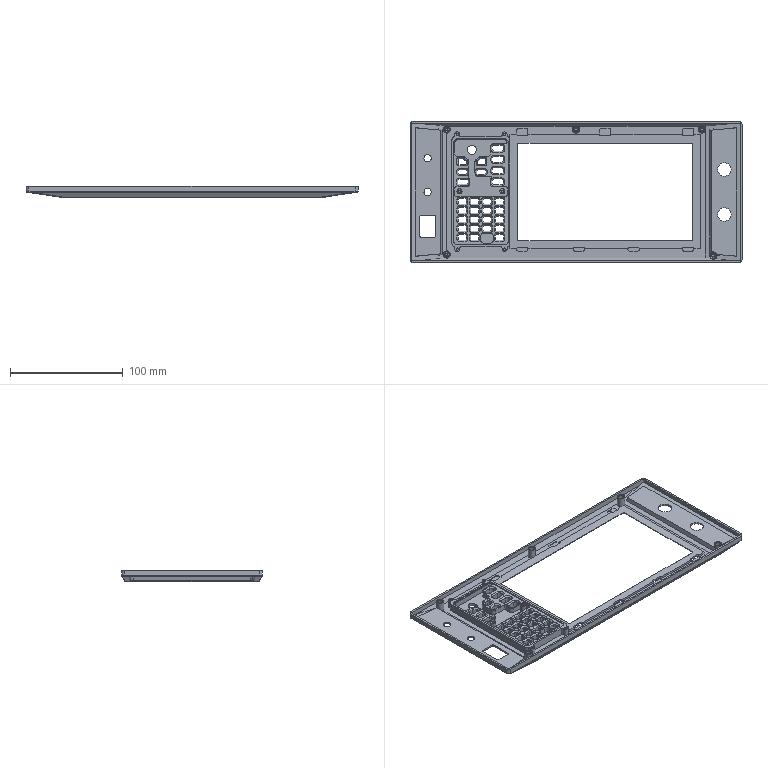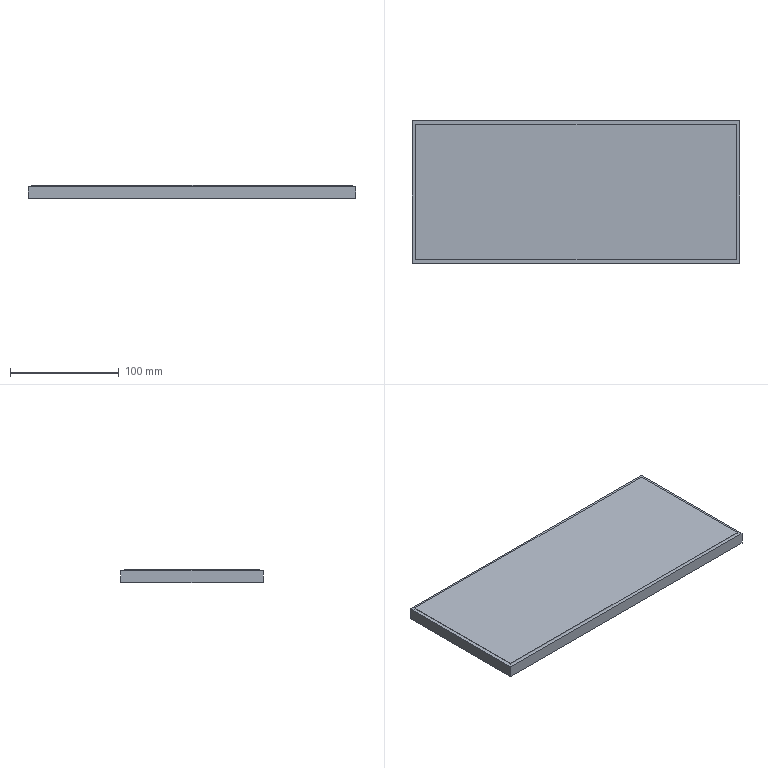CAM job | NX | 3-axis milling, drilling | part box 295 x 125 x 10 mm | stock box 301 x 131 x 12 mm
Tools:
number,name,description,diameter,corner_radius,flute_length,length,flutes
1,D63,Milling Tool-5 Parameters,63.0,0.0,50.0,75.0,2
7,D6A45,Milling Tool-5 Parameters,6.0,0.0,50.0,75.0,2
12,2.5ZT,Drilling Tool,2.5,0.0,35.0,50.0,2
13,2.1ZT,Drilling Tool,2.05,0.0,35.0,50.0,2
10,D10,Milling Tool-5 Parameters,10.0,0.0,50.0,75.0,2
6,D6,Milling Tool-5 Parameters,6.0,0.0,50.0,75.0,2
4,D4,Milling Tool-5 Parameters,4.0,0.0,50.0,75.0,2
2,D2,Milling Tool-5 Parameters,2.0,0.0,50.0,75.0,2
15,D1.5,Milling Tool-5 Parameters,1.5,0.0,50.0,75.0,2
5,D2R0.5,Milling Tool-5 Parameters,2.0,0.5,50.0,75.0,2
9,D6R0.5,Milling Tool-5 Parameters,6.0,0.5,50.0,75.0,2
Operations:
program,operation,operation_type,tool,method,geometry_group,spindle_rpm,surface_speed,feed_per_tooth,feed_cut,feed_plunge,cut_length_mm,path_length_mm,cut_time_min,machine_time_min
1,FLOOR_WALL,VolumeBased25DMillingOperation,D63,METHOD,A,6500.0,1286.0,0.0962,1250.0,100.0,1573.797,1627.797,1.259,1.264
1,DRILLING,Operation,D6A45,METHOD,A,5000.0,94.0,0.025,250.0,0.0,40.0,648.236,0.16,0.2208
1,DRILLING_COPY,Operation,2.5ZT,METHOD,A,2000.0,15.0,0.03,120.0,0.0,42.0,629.23,0.35,0.4087
1,DRILLING_COPY_COPY,Operation,2.1ZT,METHOD,A,2000.0,12.0,0.03,120.0,0.0,63.0,425.557,0.525,0.5613
1,ADAPTIVE_MILLING,CavityMilling,D10,METHOD,A,9500.0,298.0,0.1579,3000.0,1000.0,3506.591,3580.591,1.171,1.178
1,ADAPTIVE_MILLING_COPY,CavityMilling,D10,METHOD,A,9500.0,298.0,0.1579,3000.0,1000.0,26947.709,27013.909,9.563,9.57
1,CAVITY_MILL,CavityMilling,D10,METHOD,A,9500.0,298.0,0.1579,3000.0,1000.0,26927.247,28801.245,10.357,10.545
1,CAVITY_MILL_COPY,CavityMilling,D6,METHOD,A,9500.0,179.0,0.1053,2000.0,1000.0,13061.75,22740.845,8.004,8.972
1,ZLEVEL_PROFILE_COPY_COPY_COPY_1,ZLevelMilling,D6,METHOD,A,9500.0,44.0,0.0526,1000.0,100.0,860.807,937.807,0.8608,0.8685
1,HOLE_MILLING,CylinderMilling,D4,METHOD,A,9500.0,119.0,0.0737,1400.0,100.0,544.282,1273.844,0.3888,0.4617
1,HOLE_MILLING_COPY,CylinderMilling,D4,METHOD,A,9500.0,119.0,0.0526,1000.0,100.0,202.496,932.058,0.2025,0.2755
1,CAVITY_MILL_COPY_COPY,CavityMilling,D4,METHOD,A,9500.0,119.0,0.0868,1650.0,1000.0,30994.875,48438.889,25.426,27.171
1,FLOOR_WALL_1,VolumeBased25DMillingOperation,D4,METHOD,A,9500.0,119.0,0.0526,1000.0,100.0,15303.61,21184.288,15.304,15.892
1,CAVITY_MILL_COPY_COPY_COPY,CavityMilling,D2,METHOD,A,9500.0,59.0,0.0526,1000.0,1000.0,51842.907,83769.591,51.843,55.036
1,HOLE_MILLING_1,CylinderMilling,D2,METHOD,A,9500.0,59.0,0.0579,1100.0,100.0,1184.848,1993.624,1.077,1.158
1,ZLEVEL_PROFILE_COPY_COPY,ZLevelMilling,D2,METHOD,A,9500.0,44.0,0.0526,1000.0,100.0,63.243,131.781,0.0632,0.0701
1,ZLEVEL_PROFILE_COPY_COPY_COPY,ZLevelMilling,D2,METHOD,A,9500.0,44.0,0.0526,1000.0,100.0,609.106,3438.851,0.6091,0.8921
1,ZLEVEL_PROFILE_COPY_COPY_COPY_2,ZLevelMilling,D2,METHOD,A,9500.0,44.0,0.0526,1000.0,100.0,480.478,553.478,0.4805,0.4878
1,CAVITY_MILL_COPY_COPY_COPY_COPY,CavityMilling,D1.5,METHOD,A,9500.0,44.0,0.0526,1000.0,1000.0,7883.378,15369.763,7.883,8.632
1,ZLEVEL_PROFILE,ZLevelMilling,D1.5,METHOD,A,9500.0,44.0,0.0526,1000.0,100.0,825.938,886.652,0.8259,0.832
1,ZLEVEL_PROFILE_COPY,ZLevelMilling,D1.5,METHOD,A,9500.0,44.0,0.0526,1000.0,100.0,571.167,1165.156,0.5712,0.6306
1,ZLEVEL_PROFILE_1,ZLevelMilling,D2R0.5,METHOD,A,9500.0,59.0,0.1158,2200.0,1000.0,21046.46,28145.882,9.651,10.361
1,ZLEVEL_PROFILE_1_COPY,ZLevelMilling,D2R0.5,METHOD,A,9500.0,59.0,0.1158,2200.0,1000.0,18059.626,23137.615,8.265,8.773
1,ZLEVEL_PROFILE_1_COPY_COPY,ZLevelMilling,D2R0.5,METHOD,A,9500.0,59.0,0.1158,2200.0,1000.0,8241.008,8706.272,3.749,3.795
1,ZLEVEL_PROFILE_1_COPY_COPY_COPY,ZLevelMilling,D2R0.5,METHOD,A,9500.0,59.0,0.1158,2200.0,1000.0,12991.833,16669.443,5.961,6.329
1,PLANAR_MILL,PlanarMilling,D6A45,METHOD,A,9500.0,179.0,0.0658,1250.0,100.0,1678.266,2105.707,1.343,1.385
2,FLOOR_WALL_COPY,VolumeBased25DMillingOperation,D63,METHOD,B,6500.0,1286.0,0.0962,1250.0,100.0,2371.594,2855.027,1.897,1.946
2,ZLEVEL_PROFILE_1_COPY_1,ZLevelMilling,D10,METHOD,B,9500.0,179.0,0.1158,2200.0,1000.0,1080.96,1139.86,0.5171,0.523
2,FLOOR_WALL_2,VolumeBased25DMillingOperation,D6,METHOD,B,9500.0,298.0,0.1316,2500.0,1000.0,11036.893,11605.572,4.465,4.522
2,FLOOR_WALL_1_COPY,VolumeBased25DMillingOperation,D6,METHOD,B,9500.0,119.0,0.0526,1000.0,100.0,2640.621,3454.062,2.641,2.722
2,ZLEVEL_PROFILE_1_COPY_COPY_COPY_COPY_COPY_COPY,ZLevelMilling,D6,METHOD,B,9500.0,179.0,0.1053,2000.0,1000.0,161.655,968.896,0.0992,0.1799
2,FLOOR_WALL_1_COPY_COPY,VolumeBased25DMillingOperation,D6,METHOD,B,9500.0,119.0,0.0526,1000.0,100.0,514.438,575.438,0.5144,0.5205
2,ZLEVEL_PROFILE_1_COPY_COPY_COPY_COPY,ZLevelMilling,D6R0.5,METHOD,MCS_MILL_B,9500.0,179.0,0.1579,3000.0,1000.0,268763.552,268826.76,89.59,89.596
2,ZLEVEL_PROFILE_1_COPY_COPY_COPY_COPY_1,ZLevelMilling,D6R0.5,METHOD,B,9500.0,179.0,0.1579,3000.0,1000.0,8847.233,9261.269,2.953,2.995
2,ZLEVEL_PROFILE_1_COPY_COPY_COPY_COPY_COPY_COPY_COPY,ZLevelMilling,D4,METHOD,B,9500.0,119.0,0.0842,1600.0,1000.0,101.453,903.078,0.0726,0.1527
2,ZLEVEL_PROFILE_1_COPY_COPY_COPY_COPY_COPY_COPY_COPY_COPY,ZLevelMilling,D2,METHOD,B,9500.0,59.0,0.0632,1200.0,1000.0,168.823,1023.811,0.1451,0.2306
2,ZLEVEL_PROFILE_1_COPY_COPY_COPY_COPY_COPY,ZLevelMilling,D2R0.5,METHOD,B,9500.0,179.0,0.1579,3000.0,1000.0,18009.118,18134.749,6.006,6.018
2,ZLEVEL_PROFILE_COPY_1,ZLevelMilling,D6A45,METHOD,B,9500.0,179.0,0.0526,1000.0,100.0,1185.741,3970.163,1.186,1.464